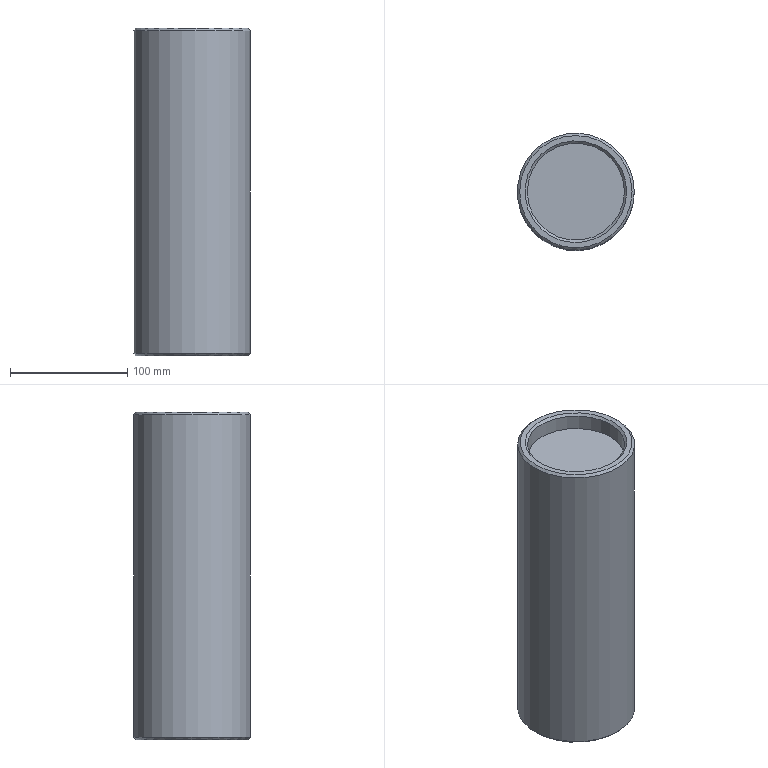Part | STEP file | lll_id4102_x_t | 1 solid | 11 faces | box 100 x 100 x 280 mm | volume 2034497 mm3 | plane 4 | cone 4 | cylinder 3 | commonest cylinder face diameters 83 x2 100 x1
STEP:
#1=CARTESIAN_POINT('',(3970.435,675.,-372.));
#2=VERTEX_POINT('',#1);
#3=CARTESIAN_POINT('',(3922.435,675.,-372.));
#4=DIRECTION('',(0.,0.,-1.));
#5=DIRECTION('',(1.,0.,0.));
#6=AXIS2_PLACEMENT_3D('',#3,#4,#5);
#7=CIRCLE('',#6,48.);
#8=EDGE_CURVE('',#2,#2,#7,.T.);
#9=ORIENTED_EDGE('',*,*,#8,.T.);
#10=EDGE_LOOP('',(#9));
#11=FACE_BOUND('',#10,.T.);
#12=CARTESIAN_POINT('',(3965.935,675.,-372.));
#13=VERTEX_POINT('',#12);
#14=CARTESIAN_POINT('',(3922.435,675.,-372.));
#15=DIRECTION('',(0.,0.,1.));
#16=DIRECTION('',(1.,0.,0.));
#17=AXIS2_PLACEMENT_3D('',#14,#15,#16);
#18=CIRCLE('',#17,43.5);
#19=EDGE_CURVE('',#13,#13,#18,.T.);
#20=ORIENTED_EDGE('',*,*,#19,.T.);
#21=EDGE_LOOP('',(#20));
#22=FACE_BOUND('',#21,.T.);
#23=CARTESIAN_POINT('',(3922.435,675.,-372.));
#24=DIRECTION('',(0.,0.,-1.));
#25=DIRECTION('',(1.,0.,0.));
#26=AXIS2_PLACEMENT_3D('',#23,#24,#25);
#27=PLANE('',#26);
#28=ADVANCED_FACE('',(#11,#22),#27,.T.);
#29=CARTESIAN_POINT('',(3970.435,675.,-92.));
#30=VERTEX_POINT('',#29);
#31=CARTESIAN_POINT('',(3922.435,675.,-92.));
#32=DIRECTION('',(0.,0.,1.));
#33=DIRECTION('',(1.,0.,0.));
#34=AXIS2_PLACEMENT_3D('',#31,#32,#33);
#35=CIRCLE('',#34,48.);
#36=EDGE_CURVE('',#30,#30,#35,.T.);
#37=ORIENTED_EDGE('',*,*,#36,.T.);
#38=EDGE_LOOP('',(#37));
#39=FACE_BOUND('',#38,.T.);
#40=CARTESIAN_POINT('',(3965.935,675.,-92.));
#41=VERTEX_POINT('',#40);
#42=CARTESIAN_POINT('',(3922.435,675.,-92.));
#43=DIRECTION('',(0.,0.,-1.));
#44=DIRECTION('',(1.,0.,0.));
#45=AXIS2_PLACEMENT_3D('',#42,#43,#44);
#46=CIRCLE('',#45,43.5);
#47=EDGE_CURVE('',#41,#41,#46,.T.);
#48=ORIENTED_EDGE('',*,*,#47,.T.);
#49=EDGE_LOOP('',(#48));
#50=FACE_BOUND('',#49,.T.);
#51=CARTESIAN_POINT('',(3922.435,675.,-92.));
#52=DIRECTION('',(0.,0.,-1.));
#53=DIRECTION('',(1.,0.,0.));
#54=AXIS2_PLACEMENT_3D('',#51,#52,#53);
#55=PLANE('',#54);
#56=ADVANCED_FACE('',(#39,#50),#55,.F.);
#57=CARTESIAN_POINT('',(3972.435,675.,-94.));
#58=VERTEX_POINT('',#57);
#59=CARTESIAN_POINT('',(3922.435,675.,-94.));
#60=DIRECTION('',(0.,0.,-1.));
#61=DIRECTION('',(1.,0.,0.));
#62=AXIS2_PLACEMENT_3D('',#59,#60,#61);
#63=CIRCLE('',#62,50.);
#64=EDGE_CURVE('',#58,#58,#63,.T.);
#65=ORIENTED_EDGE('',*,*,#64,.T.);
#66=EDGE_LOOP('',(#65));
#67=FACE_BOUND('',#66,.T.);
#68=CARTESIAN_POINT('',(3972.435,675.,-370.));
#69=VERTEX_POINT('',#68);
#70=CARTESIAN_POINT('',(3922.435,675.,-370.));
#71=DIRECTION('',(0.,0.,1.));
#72=DIRECTION('',(1.,0.,0.));
#73=AXIS2_PLACEMENT_3D('',#70,#71,#72);
#74=CIRCLE('',#73,50.);
#75=EDGE_CURVE('',#69,#69,#74,.T.);
#76=ORIENTED_EDGE('',*,*,#75,.T.);
#77=EDGE_LOOP('',(#76));
#78=FACE_BOUND('',#77,.T.);
#79=CARTESIAN_POINT('',(3922.435,675.,-107.));
#80=DIRECTION('',(0.,0.,-1.));
#81=DIRECTION('',(1.,0.,0.));
#82=AXIS2_PLACEMENT_3D('',#79,#80,#81);
#83=CYLINDRICAL_SURFACE('',#82,50.);
#84=ADVANCED_FACE('',(#67,#78),#83,.T.);
#85=CARTESIAN_POINT('',(3963.935,675.,-94.));
#86=VERTEX_POINT('',#85);
#87=CARTESIAN_POINT('',(3922.435,675.,-94.));
#88=DIRECTION('',(0.,0.,1.));
#89=DIRECTION('',(1.,0.,0.));
#90=AXIS2_PLACEMENT_3D('',#87,#88,#89);
#91=CIRCLE('',#90,41.5);
#92=EDGE_CURVE('',#86,#86,#91,.T.);
#93=ORIENTED_EDGE('',*,*,#92,.T.);
#94=EDGE_LOOP('',(#93));
#95=FACE_BOUND('',#94,.T.);
#96=CARTESIAN_POINT('',(3963.935,675.,-107.));
#97=VERTEX_POINT('',#96);
#98=CARTESIAN_POINT('',(3922.435,675.,-107.));
#99=DIRECTION('',(0.,0.,1.));
#100=DIRECTION('',(1.,0.,0.));
#101=AXIS2_PLACEMENT_3D('',#98,#99,#100);
#102=CIRCLE('',#101,41.5);
#103=EDGE_CURVE('',#97,#97,#102,.T.);
#104=ORIENTED_EDGE('',*,*,#103,.F.);
#105=EDGE_LOOP('',(#104));
#106=FACE_BOUND('',#105,.T.);
#107=CARTESIAN_POINT('',(3922.435,675.,-92.));
#108=DIRECTION('',(0.,0.,-1.));
#109=DIRECTION('',(1.,0.,0.));
#110=AXIS2_PLACEMENT_3D('',#107,#108,#109);
#111=CYLINDRICAL_SURFACE('',#110,41.5);
#112=ADVANCED_FACE('',(#95,#106),#111,.F.);
#113=ORIENTED_EDGE('',*,*,#103,.T.);
#114=EDGE_LOOP('',(#113));
#115=FACE_OUTER_BOUND('',#114,.T.);
#116=CARTESIAN_POINT('',(3922.435,675.,-107.));
#117=DIRECTION('',(0.,0.,-1.));
#118=DIRECTION('',(1.,0.,0.));
#119=AXIS2_PLACEMENT_3D('',#116,#117,#118);
#120=PLANE('',#119);
#121=ADVANCED_FACE('',(#115),#120,.F.);
#122=CARTESIAN_POINT('',(3963.935,675.,-370.));
#123=VERTEX_POINT('',#122);
#124=CARTESIAN_POINT('',(3922.435,675.,-370.));
#125=DIRECTION('',(0.,0.,-1.));
#126=DIRECTION('',(1.,0.,0.));
#127=AXIS2_PLACEMENT_3D('',#124,#125,#126);
#128=CIRCLE('',#127,41.5);
#129=EDGE_CURVE('',#123,#123,#128,.T.);
#130=ORIENTED_EDGE('',*,*,#129,.T.);
#131=EDGE_LOOP('',(#130));
#132=FACE_BOUND('',#131,.T.);
#133=CARTESIAN_POINT('',(3963.935,675.,-357.));
#134=VERTEX_POINT('',#133);
#135=CARTESIAN_POINT('',(3922.435,675.,-357.));
#136=DIRECTION('',(0.,0.,-1.));
#137=DIRECTION('',(1.,0.,0.));
#138=AXIS2_PLACEMENT_3D('',#135,#136,#137);
#139=CIRCLE('',#138,41.5);
#140=EDGE_CURVE('',#134,#134,#139,.T.);
#141=ORIENTED_EDGE('',*,*,#140,.F.);
#142=EDGE_LOOP('',(#141));
#143=FACE_BOUND('',#142,.T.);
#144=CARTESIAN_POINT('',(3922.435,675.,-372.));
#145=DIRECTION('',(0.,0.,1.));
#146=DIRECTION('',(-1.,0.,0.));
#147=AXIS2_PLACEMENT_3D('',#144,#145,#146);
#148=CYLINDRICAL_SURFACE('',#147,41.5);
#149=ADVANCED_FACE('',(#132,#143),#148,.F.);
#150=ORIENTED_EDGE('',*,*,#140,.T.);
#151=EDGE_LOOP('',(#150));
#152=FACE_OUTER_BOUND('',#151,.T.);
#153=CARTESIAN_POINT('',(3922.435,675.,-357.));
#154=DIRECTION('',(0.,0.,1.));
#155=DIRECTION('',(-1.,0.,0.));
#156=AXIS2_PLACEMENT_3D('',#153,#154,#155);
#157=PLANE('',#156);
#158=ADVANCED_FACE('',(#152),#157,.F.);
#159=ORIENTED_EDGE('',*,*,#36,.F.);
#160=EDGE_LOOP('',(#159));
#161=FACE_BOUND('',#160,.T.);
#162=ORIENTED_EDGE('',*,*,#64,.F.);
#163=EDGE_LOOP('',(#162));
#164=FACE_BOUND('',#163,.T.);
#165=CARTESIAN_POINT('',(3922.435,675.,-94.));
#166=DIRECTION('',(0.,0.,-1.));
#167=DIRECTION('',(1.,0.,0.));
#168=AXIS2_PLACEMENT_3D('',#165,#166,#167);
#169=CONICAL_SURFACE('',#168,50.,45.);
#170=ADVANCED_FACE('',(#161,#164),#169,.T.);
#171=ORIENTED_EDGE('',*,*,#92,.F.);
#172=EDGE_LOOP('',(#171));
#173=FACE_BOUND('',#172,.T.);
#174=ORIENTED_EDGE('',*,*,#47,.F.);
#175=EDGE_LOOP('',(#174));
#176=FACE_BOUND('',#175,.T.);
#177=CARTESIAN_POINT('',(3922.435,675.,-92.));
#178=DIRECTION('',(0.,0.,1.));
#179=DIRECTION('',(-1.,0.,0.));
#180=AXIS2_PLACEMENT_3D('',#177,#178,#179);
#181=CONICAL_SURFACE('',#180,43.5,45.);
#182=ADVANCED_FACE('',(#173,#176),#181,.F.);
#183=ORIENTED_EDGE('',*,*,#8,.F.);
#184=EDGE_LOOP('',(#183));
#185=FACE_BOUND('',#184,.T.);
#186=ORIENTED_EDGE('',*,*,#75,.F.);
#187=EDGE_LOOP('',(#186));
#188=FACE_BOUND('',#187,.T.);
#189=CARTESIAN_POINT('',(3922.435,675.,-370.));
#190=DIRECTION('',(0.,0.,1.));
#191=DIRECTION('',(-1.,0.,0.));
#192=AXIS2_PLACEMENT_3D('',#189,#190,#191);
#193=CONICAL_SURFACE('',#192,50.,45.);
#194=ADVANCED_FACE('',(#185,#188),#193,.T.);
#195=ORIENTED_EDGE('',*,*,#129,.F.);
#196=EDGE_LOOP('',(#195));
#197=FACE_BOUND('',#196,.T.);
#198=ORIENTED_EDGE('',*,*,#19,.F.);
#199=EDGE_LOOP('',(#198));
#200=FACE_BOUND('',#199,.T.);
#201=CARTESIAN_POINT('',(3922.435,675.,-372.));
#202=DIRECTION('',(0.,0.,-1.));
#203=DIRECTION('',(1.,0.,0.));
#204=AXIS2_PLACEMENT_3D('',#201,#202,#203);
#205=CONICAL_SURFACE('',#204,43.5,45.);
#206=ADVANCED_FACE('',(#197,#200),#205,.F.);
#207=CLOSED_SHELL('',(#28,#56,#84,#112,#121,#149,#158,#170,#182,#194,#206));
#208=MANIFOLD_SOLID_BREP('',#207);
#209=(LENGTH_UNIT()NAMED_UNIT(*)SI_UNIT(.MILLI.,.METRE.));
#210=UNCERTAINTY_MEASURE_WITH_UNIT(LENGTH_MEASURE(0.00002),#209,'','');
#211=(NAMED_UNIT(*)PLANE_ANGLE_UNIT()SI_UNIT($,.RADIAN.));
#212=PLANE_ANGLE_MEASURE_WITH_UNIT(PLANE_ANGLE_MEASURE(0.01745),#211);
#213=DIMENSIONAL_EXPONENTS(0.,0.,0.,0.,0.,0.,0.);
#214=(CONVERSION_BASED_UNIT('DEGREE',#212)NAMED_UNIT(#213)PLANE_ANGLE_UNIT());
#215=(NAMED_UNIT(*)SI_UNIT($,.STERADIAN.)SOLID_ANGLE_UNIT());
#216=(GEOMETRIC_REPRESENTATION_CONTEXT(3)GLOBAL_UNCERTAINTY_ASSIGNED_CONTEXT((#210))GLOBAL_UNIT_ASSIGNED_CONTEXT((#209,#214,#215))REPRESENTATION_CONTEXT('',''));
#217=ADVANCED_BREP_SHAPE_REPRESENTATION('',(#208),#216);